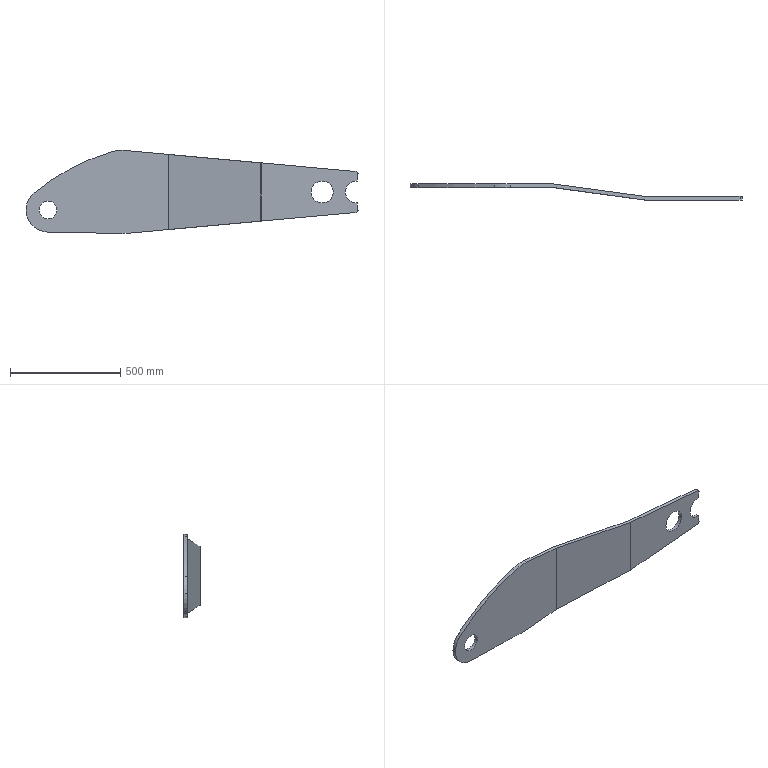Part | SolidWorks | features Extrusion 1, ICE 1 | 1 solid | 28 faces | box 1506 x 73 x 377 mm | volume 6517874 mm3 | cylinder 17 | plane 11 | commonest cylinder face diameters 20 x4 100 x4 52 x2 80 x2 200 x2 377 x2
STEP:
#1=CARTESIAN_POINT('',(-549.379,-8.,118.522));
#2=VERTEX_POINT('',#1);
#3=CARTESIAN_POINT('',(-647.3,-8.,218.5));
#4=VERTEX_POINT('',#3);
#5=CARTESIAN_POINT('',(-547.3,-8.,218.5));
#6=DIRECTION('',(0.,1.,0.));
#7=DIRECTION('',(-1.,0.,0.));
#8=AXIS2_PLACEMENT_3D('',#5,#6,#7);
#9=CIRCLE('',#8,100.);
#10=EDGE_CURVE('',#2,#4,#9,.T.);
#11=ORIENTED_EDGE('',*,*,#10,.T.);
#12=CARTESIAN_POINT('',(-647.3,8.,218.5));
#13=VERTEX_POINT('',#12);
#14=CARTESIAN_POINT('',(-647.3,-65.,218.5));
#15=DIRECTION('',(0.,1.,0.));
#16=VECTOR('',#15,1000.);
#17=LINE('',#14,#16);
#18=EDGE_CURVE('',#4,#13,#17,.T.);
#19=ORIENTED_EDGE('',*,*,#18,.T.);
#20=CARTESIAN_POINT('',(-549.379,8.,118.522));
#21=VERTEX_POINT('',#20);
#22=CARTESIAN_POINT('',(-547.3,8.,218.5));
#23=DIRECTION('',(0.,1.,0.));
#24=DIRECTION('',(-1.,0.,0.));
#25=AXIS2_PLACEMENT_3D('',#22,#23,#24);
#26=CIRCLE('',#25,100.);
#27=EDGE_CURVE('',#21,#13,#26,.T.);
#28=ORIENTED_EDGE('',*,*,#27,.F.);
#29=CARTESIAN_POINT('',(-549.379,-65.,118.522));
#30=DIRECTION('',(0.,1.,0.));
#31=VECTOR('',#30,1000.);
#32=LINE('',#29,#31);
#33=EDGE_CURVE('',#2,#21,#32,.T.);
#34=ORIENTED_EDGE('',*,*,#33,.F.);
#35=EDGE_LOOP('',(#11,#19,#28,#34));
#36=FACE_OUTER_BOUND('',#35,.T.);
#37=CARTESIAN_POINT('',(-547.3,-65.,218.5));
#38=DIRECTION('',(0.,1.,0.));
#39=DIRECTION('',(-1.,0.,0.));
#40=AXIS2_PLACEMENT_3D('',#37,#38,#39);
#41=CYLINDRICAL_SURFACE('',#40,100.);
#42=ADVANCED_FACE('',(#36),#41,.T.);
#43=CARTESIAN_POINT('',(855.554,-65.,349.792));
#44=VERTEX_POINT('',#43);
#45=CARTESIAN_POINT('',(801.,-65.,300.));
#46=VERTEX_POINT('',#45);
#47=CARTESIAN_POINT('',(851.,-65.,300.));
#48=DIRECTION('',(0.,-1.,0.));
#49=DIRECTION('',(-1.,0.,0.));
#50=AXIS2_PLACEMENT_3D('',#47,#48,#49);
#51=CIRCLE('',#50,50.);
#52=EDGE_CURVE('',#44,#46,#51,.T.);
#53=ORIENTED_EDGE('',*,*,#52,.T.);
#54=CARTESIAN_POINT('',(801.,-49.,300.));
#55=VERTEX_POINT('',#54);
#56=CARTESIAN_POINT('',(801.,-65.,300.));
#57=DIRECTION('',(0.,1.,0.));
#58=VECTOR('',#57,1000.);
#59=LINE('',#56,#58);
#60=EDGE_CURVE('',#46,#55,#59,.T.);
#61=ORIENTED_EDGE('',*,*,#60,.T.);
#62=CARTESIAN_POINT('',(855.554,-49.,349.792));
#63=VERTEX_POINT('',#62);
#64=CARTESIAN_POINT('',(851.,-49.,300.));
#65=DIRECTION('',(0.,1.,0.));
#66=DIRECTION('',(0.,0.,-1.));
#67=AXIS2_PLACEMENT_3D('',#64,#65,#66);
#68=CIRCLE('',#67,50.);
#69=EDGE_CURVE('',#55,#63,#68,.T.);
#70=ORIENTED_EDGE('',*,*,#69,.T.);
#71=CARTESIAN_POINT('',(855.554,-65.,349.792));
#72=DIRECTION('',(0.,1.,0.));
#73=VECTOR('',#72,1000.);
#74=LINE('',#71,#73);
#75=EDGE_CURVE('',#44,#63,#74,.T.);
#76=ORIENTED_EDGE('',*,*,#75,.F.);
#77=EDGE_LOOP('',(#53,#61,#70,#76));
#78=FACE_OUTER_BOUND('',#77,.T.);
#79=CARTESIAN_POINT('',(851.,-65.,300.));
#80=DIRECTION('',(0.,1.,0.));
#81=DIRECTION('',(-1.,0.,0.));
#82=AXIS2_PLACEMENT_3D('',#79,#80,#81);
#83=CYLINDRICAL_SURFACE('',#82,50.);
#84=ADVANCED_FACE('',(#78),#83,.F.);
#85=CARTESIAN_POINT('',(746.,-65.,300.));
#86=VERTEX_POINT('',#85);
#87=CARTESIAN_POINT('',(646.,-65.,300.));
#88=VERTEX_POINT('',#87);
#89=CARTESIAN_POINT('',(696.,-65.,300.));
#90=DIRECTION('',(0.,1.,0.));
#91=DIRECTION('',(-1.,0.,0.));
#92=AXIS2_PLACEMENT_3D('',#89,#90,#91);
#93=CIRCLE('',#92,50.);
#94=EDGE_CURVE('',#86,#88,#93,.T.);
#95=ORIENTED_EDGE('',*,*,#94,.F.);
#96=CARTESIAN_POINT('',(746.,-49.,300.));
#97=VERTEX_POINT('',#96);
#98=CARTESIAN_POINT('',(746.,-65.,300.));
#99=DIRECTION('',(0.,1.,0.));
#100=VECTOR('',#99,1000.);
#101=LINE('',#98,#100);
#102=EDGE_CURVE('',#86,#97,#101,.T.);
#103=ORIENTED_EDGE('',*,*,#102,.T.);
#104=CARTESIAN_POINT('',(646.,-49.,300.));
#105=VERTEX_POINT('',#104);
#106=CARTESIAN_POINT('',(696.,-49.,300.));
#107=DIRECTION('',(0.,-1.,0.));
#108=DIRECTION('',(0.,0.,-1.));
#109=AXIS2_PLACEMENT_3D('',#106,#107,#108);
#110=CIRCLE('',#109,50.);
#111=EDGE_CURVE('',#105,#97,#110,.T.);
#112=ORIENTED_EDGE('',*,*,#111,.F.);
#113=CARTESIAN_POINT('',(646.,-65.,300.));
#114=DIRECTION('',(0.,1.,0.));
#115=VECTOR('',#114,1000.);
#116=LINE('',#113,#115);
#117=EDGE_CURVE('',#88,#105,#116,.T.);
#118=ORIENTED_EDGE('',*,*,#117,.F.);
#119=EDGE_LOOP('',(#95,#103,#112,#118));
#120=FACE_OUTER_BOUND('',#119,.T.);
#121=CARTESIAN_POINT('',(696.,-65.,300.));
#122=DIRECTION('',(0.,1.,0.));
#123=DIRECTION('',(-1.,0.,0.));
#124=AXIS2_PLACEMENT_3D('',#121,#122,#123);
#125=CYLINDRICAL_SURFACE('',#124,50.);
#126=ADVANCED_FACE('',(#120),#125,.F.);
#127=CARTESIAN_POINT('',(-507.3,-8.,218.5));
#128=VERTEX_POINT('',#127);
#129=CARTESIAN_POINT('',(-587.3,-8.,218.5));
#130=VERTEX_POINT('',#129);
#131=CARTESIAN_POINT('',(-547.3,-8.,218.5));
#132=DIRECTION('',(0.,1.,0.));
#133=DIRECTION('',(-1.,0.,0.));
#134=AXIS2_PLACEMENT_3D('',#131,#132,#133);
#135=CIRCLE('',#134,40.);
#136=EDGE_CURVE('',#128,#130,#135,.T.);
#137=ORIENTED_EDGE('',*,*,#136,.F.);
#138=CARTESIAN_POINT('',(-507.3,8.,218.5));
#139=VERTEX_POINT('',#138);
#140=CARTESIAN_POINT('',(-507.3,-65.,218.5));
#141=DIRECTION('',(0.,1.,0.));
#142=VECTOR('',#141,1000.);
#143=LINE('',#140,#142);
#144=EDGE_CURVE('',#128,#139,#143,.T.);
#145=ORIENTED_EDGE('',*,*,#144,.T.);
#146=CARTESIAN_POINT('',(-587.3,8.,218.5));
#147=VERTEX_POINT('',#146);
#148=CARTESIAN_POINT('',(-547.3,8.,218.5));
#149=DIRECTION('',(0.,1.,0.));
#150=DIRECTION('',(-1.,0.,0.));
#151=AXIS2_PLACEMENT_3D('',#148,#149,#150);
#152=CIRCLE('',#151,40.);
#153=EDGE_CURVE('',#139,#147,#152,.T.);
#154=ORIENTED_EDGE('',*,*,#153,.T.);
#155=CARTESIAN_POINT('',(-587.3,-65.,218.5));
#156=DIRECTION('',(0.,1.,0.));
#157=VECTOR('',#156,1000.);
#158=LINE('',#155,#157);
#159=EDGE_CURVE('',#130,#147,#158,.T.);
#160=ORIENTED_EDGE('',*,*,#159,.F.);
#161=EDGE_LOOP('',(#137,#145,#154,#160));
#162=FACE_OUTER_BOUND('',#161,.T.);
#163=CARTESIAN_POINT('',(-547.3,-65.,218.5));
#164=DIRECTION('',(0.,1.,0.));
#165=DIRECTION('',(-1.,0.,0.));
#166=AXIS2_PLACEMENT_3D('',#163,#164,#165);
#167=CYLINDRICAL_SURFACE('',#166,40.);
#168=ADVANCED_FACE('',(#162),#167,.F.);
#169=CARTESIAN_POINT('',(-1.216,-8.,470.323));
#170=VERTEX_POINT('',#169);
#171=CARTESIAN_POINT('',(0.129,-8.091,470.2));
#172=VERTEX_POINT('',#171);
#173=CARTESIAN_POINT('',(-1.216,-8.,470.323));
#174=CARTESIAN_POINT('',(-0.7662,-8.,470.282));
#175=CARTESIAN_POINT('',(-0.3171,-8.03,470.241));
#176=CARTESIAN_POINT('',(0.129,-8.091,470.2));
#177=(BOUNDED_CURVE()B_SPLINE_CURVE(3,(#173,#174,#175,#176),.UNSPECIFIED.,.F.,.T.)B_SPLINE_CURVE_WITH_KNOTS((4,4),(4.712,4.847),.UNSPECIFIED.)CURVE()GEOMETRIC_REPRESENTATION_ITEM()RATIONAL_B_SPLINE_CURVE((1.,0.9985,0.9985,1.))REPRESENTATION_ITEM(''));
#178=EDGE_CURVE('',#170,#172,#177,.T.);
#179=ORIENTED_EDGE('',*,*,#178,.F.);
#180=CARTESIAN_POINT('',(-1.216,-8.,129.677));
#181=VERTEX_POINT('',#180);
#182=CARTESIAN_POINT('',(-1.216,-8.,600.));
#183=DIRECTION('',(0.,0.,-1.));
#184=VECTOR('',#183,1000.);
#185=LINE('',#182,#184);
#186=EDGE_CURVE('',#170,#181,#185,.T.);
#187=ORIENTED_EDGE('',*,*,#186,.T.);
#188=CARTESIAN_POINT('',(0.129,-8.091,129.8));
#189=VERTEX_POINT('',#188);
#190=CARTESIAN_POINT('',(0.129,-8.091,129.8));
#191=CARTESIAN_POINT('',(-0.3171,-8.03,129.759));
#192=CARTESIAN_POINT('',(-0.7662,-8.,129.718));
#193=CARTESIAN_POINT('',(-1.216,-8.,129.677));
#194=(BOUNDED_CURVE()B_SPLINE_CURVE(3,(#190,#191,#192,#193),.UNSPECIFIED.,.F.,.T.)B_SPLINE_CURVE_WITH_KNOTS((4,4),(4.577,4.712),.UNSPECIFIED.)CURVE()GEOMETRIC_REPRESENTATION_ITEM()RATIONAL_B_SPLINE_CURVE((1.,0.9985,0.9985,1.))REPRESENTATION_ITEM(''));
#195=EDGE_CURVE('',#189,#181,#194,.T.);
#196=ORIENTED_EDGE('',*,*,#195,.F.);
#197=CARTESIAN_POINT('',(0.129,-8.091,600.));
#198=DIRECTION('',(0.,0.,-1.));
#199=VECTOR('',#198,1000.);
#200=LINE('',#197,#199);
#201=EDGE_CURVE('',#172,#189,#200,.T.);
#202=ORIENTED_EDGE('',*,*,#201,.F.);
#203=EDGE_LOOP('',(#179,#187,#196,#202));
#204=FACE_OUTER_BOUND('',#203,.T.);
#205=CARTESIAN_POINT('',(-1.216,-18.,600.));
#206=DIRECTION('',(0.,0.,-1.));
#207=DIRECTION('',(-1.,0.,0.));
#208=AXIS2_PLACEMENT_3D('',#205,#206,#207);
#209=CYLINDRICAL_SURFACE('',#208,10.);
#210=ADVANCED_FACE('',(#204),#209,.F.);
#211=CARTESIAN_POINT('',(417.518,-64.764,432.272));
#212=VERTEX_POINT('',#211);
#213=CARTESIAN_POINT('',(-11.359,-6.531,471.244));
#214=DIRECTION('',(0.9869,-0.134,-0.08968));
#215=VECTOR('',#214,1000.);
#216=LINE('',#213,#215);
#217=EDGE_CURVE('',#172,#212,#216,.T.);
#218=ORIENTED_EDGE('',*,*,#217,.F.);
#219=ORIENTED_EDGE('',*,*,#201,.T.);
#220=CARTESIAN_POINT('',(417.518,-64.764,167.728));
#221=VERTEX_POINT('',#220);
#222=CARTESIAN_POINT('',(41.746,-13.742,133.581));
#223=DIRECTION('',(-0.9869,0.134,-0.08968));
#224=VECTOR('',#223,1000.);
#225=LINE('',#222,#224);
#226=EDGE_CURVE('',#221,#189,#225,.T.);
#227=ORIENTED_EDGE('',*,*,#226,.F.);
#228=CARTESIAN_POINT('',(417.518,-64.764,600.));
#229=DIRECTION('',(0.,0.,-1.));
#230=VECTOR('',#229,1000.);
#231=LINE('',#228,#230);
#232=EDGE_CURVE('',#212,#221,#231,.T.);
#233=ORIENTED_EDGE('',*,*,#232,.F.);
#234=EDGE_LOOP('',(#218,#219,#227,#233));
#235=FACE_OUTER_BOUND('',#234,.T.);
#236=CARTESIAN_POINT('',(0.129,-8.091,600.));
#237=DIRECTION('',(0.1345,0.9909,0.));
#238=DIRECTION('',(-0.9909,0.1345,0.));
#239=AXIS2_PLACEMENT_3D('',#236,#237,#238);
#240=PLANE('',#239);
#241=ADVANCED_FACE('',(#235),#240,.F.);
#242=CARTESIAN_POINT('',(421.016,-65.,431.954));
#243=VERTEX_POINT('',#242);
#244=CARTESIAN_POINT('',(417.518,-64.764,432.272));
#245=CARTESIAN_POINT('',(418.678,-64.921,432.166));
#246=CARTESIAN_POINT('',(419.846,-65.,432.06));
#247=CARTESIAN_POINT('',(421.016,-65.,431.954));
#248=(BOUNDED_CURVE()B_SPLINE_CURVE(3,(#244,#245,#246,#247),.UNSPECIFIED.,.F.,.T.)B_SPLINE_CURVE_WITH_KNOTS((4,4),(4.577,4.712),.UNSPECIFIED.)CURVE()GEOMETRIC_REPRESENTATION_ITEM()RATIONAL_B_SPLINE_CURVE((1.,0.9985,0.9985,1.))REPRESENTATION_ITEM(''));
#249=EDGE_CURVE('',#212,#243,#248,.T.);
#250=ORIENTED_EDGE('',*,*,#249,.F.);
#251=ORIENTED_EDGE('',*,*,#232,.T.);
#252=CARTESIAN_POINT('',(421.016,-65.,168.046));
#253=VERTEX_POINT('',#252);
#254=CARTESIAN_POINT('',(421.016,-65.,168.046));
#255=CARTESIAN_POINT('',(419.846,-65.,167.94));
#256=CARTESIAN_POINT('',(418.678,-64.921,167.834));
#257=CARTESIAN_POINT('',(417.518,-64.764,167.728));
#258=(BOUNDED_CURVE()B_SPLINE_CURVE(3,(#254,#255,#256,#257),.UNSPECIFIED.,.F.,.T.)B_SPLINE_CURVE_WITH_KNOTS((4,4),(4.712,4.847),.UNSPECIFIED.)CURVE()GEOMETRIC_REPRESENTATION_ITEM()RATIONAL_B_SPLINE_CURVE((1.,0.9985,0.9985,1.))REPRESENTATION_ITEM(''));
#259=EDGE_CURVE('',#253,#221,#258,.T.);
#260=ORIENTED_EDGE('',*,*,#259,.F.);
#261=CARTESIAN_POINT('',(421.016,-65.,600.));
#262=DIRECTION('',(0.,0.,-1.));
#263=VECTOR('',#262,1000.);
#264=LINE('',#261,#263);
#265=EDGE_CURVE('',#243,#253,#264,.T.);
#266=ORIENTED_EDGE('',*,*,#265,.F.);
#267=EDGE_LOOP('',(#250,#251,#260,#266));
#268=FACE_OUTER_BOUND('',#267,.T.);
#269=CARTESIAN_POINT('',(421.016,-39.,600.));
#270=DIRECTION('',(0.,0.,-1.));
#271=DIRECTION('',(-1.,0.,0.));
#272=AXIS2_PLACEMENT_3D('',#269,#270,#271);
#273=CYLINDRICAL_SURFACE('',#272,26.);
#274=ADVANCED_FACE('',(#268),#273,.T.);
#275=CARTESIAN_POINT('',(696.,-65.,300.));
#276=DIRECTION('',(0.,1.,0.));
#277=DIRECTION('',(-1.,0.,0.));
#278=AXIS2_PLACEMENT_3D('',#275,#276,#277);
#279=CIRCLE('',#278,50.);
#280=EDGE_CURVE('',#88,#86,#279,.T.);
#281=ORIENTED_EDGE('',*,*,#280,.T.);
#282=ORIENTED_EDGE('',*,*,#94,.T.);
#283=EDGE_LOOP('',(#281,#282));
#284=FACE_BOUND('',#283,.T.);
#285=CARTESIAN_POINT('',(849.441,-65.,393.023));
#286=VERTEX_POINT('',#285);
#287=CARTESIAN_POINT('',(849.441,-65.,393.023));
#288=DIRECTION('',(0.9959,0.,-0.0905));
#289=VECTOR('',#288,1000.);
#290=LINE('',#287,#289);
#291=EDGE_CURVE('',#243,#286,#290,.T.);
#292=ORIENTED_EDGE('',*,*,#291,.F.);
#293=ORIENTED_EDGE('',*,*,#265,.T.);
#294=CARTESIAN_POINT('',(849.441,-65.,206.977));
#295=VERTEX_POINT('',#294);
#296=CARTESIAN_POINT('',(849.441,-65.,206.977));
#297=DIRECTION('',(-0.9959,0.,-0.0905));
#298=VECTOR('',#297,1000.);
#299=LINE('',#296,#298);
#300=EDGE_CURVE('',#295,#253,#299,.T.);
#301=ORIENTED_EDGE('',*,*,#300,.F.);
#302=CARTESIAN_POINT('',(858.495,-65.,217.841));
#303=VERTEX_POINT('',#302);
#304=CARTESIAN_POINT('',(848.536,-65.,216.936));
#305=DIRECTION('',(0.,1.,0.));
#306=DIRECTION('',(1.,0.,0.));
#307=AXIS2_PLACEMENT_3D('',#304,#305,#306);
#308=CIRCLE('',#307,10.);
#309=EDGE_CURVE('',#303,#295,#308,.T.);
#310=ORIENTED_EDGE('',*,*,#309,.F.);
#311=CARTESIAN_POINT('',(855.554,-65.,250.208));
#312=VERTEX_POINT('',#311);
#313=CARTESIAN_POINT('',(858.495,-65.,217.841));
#314=DIRECTION('',(0.0905,0.,-0.9959));
#315=VECTOR('',#314,1000.);
#316=LINE('',#313,#315);
#317=EDGE_CURVE('',#312,#303,#316,.T.);
#318=ORIENTED_EDGE('',*,*,#317,.F.);
#319=CARTESIAN_POINT('',(851.,-65.,300.));
#320=DIRECTION('',(0.,-1.,0.));
#321=DIRECTION('',(-1.,0.,0.));
#322=AXIS2_PLACEMENT_3D('',#319,#320,#321);
#323=CIRCLE('',#322,50.);
#324=EDGE_CURVE('',#46,#312,#323,.T.);
#325=ORIENTED_EDGE('',*,*,#324,.F.);
#326=ORIENTED_EDGE('',*,*,#52,.F.);
#327=CARTESIAN_POINT('',(858.495,-65.,382.159));
#328=VERTEX_POINT('',#327);
#329=CARTESIAN_POINT('',(858.495,-65.,382.159));
#330=DIRECTION('',(-0.0905,0.,-0.9959));
#331=VECTOR('',#330,1000.);
#332=LINE('',#329,#331);
#333=EDGE_CURVE('',#328,#44,#332,.T.);
#334=ORIENTED_EDGE('',*,*,#333,.F.);
#335=CARTESIAN_POINT('',(848.536,-65.,383.064));
#336=DIRECTION('',(0.,1.,0.));
#337=DIRECTION('',(-1.,0.,0.));
#338=AXIS2_PLACEMENT_3D('',#335,#336,#337);
#339=CIRCLE('',#338,10.);
#340=EDGE_CURVE('',#286,#328,#339,.T.);
#341=ORIENTED_EDGE('',*,*,#340,.F.);
#342=EDGE_LOOP('',(#292,#293,#301,#310,#318,#325,#326,#334,#341));
#343=FACE_OUTER_BOUND('',#342,.T.);
#344=CARTESIAN_POINT('',(421.016,-65.,600.));
#345=DIRECTION('',(0.,1.,0.));
#346=DIRECTION('',(-1.,0.,0.));
#347=AXIS2_PLACEMENT_3D('',#344,#345,#346);
#348=PLANE('',#347);
#349=ADVANCED_FACE('',(#284,#343),#348,.F.);
#350=ORIENTED_EDGE('',*,*,#111,.T.);
#351=CARTESIAN_POINT('',(696.,-49.,300.));
#352=DIRECTION('',(0.,-1.,0.));
#353=DIRECTION('',(0.,0.,-1.));
#354=AXIS2_PLACEMENT_3D('',#351,#352,#353);
#355=CIRCLE('',#354,50.);
#356=EDGE_CURVE('',#97,#105,#355,.T.);
#357=ORIENTED_EDGE('',*,*,#356,.T.);
#358=EDGE_LOOP('',(#350,#357));
#359=FACE_BOUND('',#358,.T.);
#360=CARTESIAN_POINT('',(849.441,-49.,393.023));
#361=VERTEX_POINT('',#360);
#362=CARTESIAN_POINT('',(421.016,-49.,431.954));
#363=VERTEX_POINT('',#362);
#364=CARTESIAN_POINT('',(405.871,-49.,433.33));
#365=DIRECTION('',(-0.9959,0.,0.0905));
#366=VECTOR('',#365,1000.);
#367=LINE('',#364,#366);
#368=EDGE_CURVE('',#361,#363,#367,.T.);
#369=ORIENTED_EDGE('',*,*,#368,.F.);
#370=CARTESIAN_POINT('',(858.495,-49.,382.159));
#371=VERTEX_POINT('',#370);
#372=CARTESIAN_POINT('',(848.536,-49.,383.064));
#373=DIRECTION('',(0.,-1.,0.));
#374=DIRECTION('',(0.,0.,-1.));
#375=AXIS2_PLACEMENT_3D('',#372,#373,#374);
#376=CIRCLE('',#375,10.);
#377=EDGE_CURVE('',#371,#361,#376,.T.);
#378=ORIENTED_EDGE('',*,*,#377,.F.);
#379=CARTESIAN_POINT('',(874.545,-49.,558.788));
#380=DIRECTION('',(0.0905,0.,0.9959));
#381=VECTOR('',#380,1000.);
#382=LINE('',#379,#381);
#383=EDGE_CURVE('',#63,#371,#382,.T.);
#384=ORIENTED_EDGE('',*,*,#383,.F.);
#385=ORIENTED_EDGE('',*,*,#69,.F.);
#386=CARTESIAN_POINT('',(855.554,-49.,250.208));
#387=VERTEX_POINT('',#386);
#388=CARTESIAN_POINT('',(851.,-49.,300.));
#389=DIRECTION('',(0.,1.,0.));
#390=DIRECTION('',(0.,0.,-1.));
#391=AXIS2_PLACEMENT_3D('',#388,#389,#390);
#392=CIRCLE('',#391,50.);
#393=EDGE_CURVE('',#387,#55,#392,.T.);
#394=ORIENTED_EDGE('',*,*,#393,.F.);
#395=CARTESIAN_POINT('',(858.495,-49.,217.841));
#396=VERTEX_POINT('',#395);
#397=CARTESIAN_POINT('',(820.47,-49.,636.299));
#398=DIRECTION('',(-0.0905,0.,0.9959));
#399=VECTOR('',#398,1000.);
#400=LINE('',#397,#399);
#401=EDGE_CURVE('',#396,#387,#400,.T.);
#402=ORIENTED_EDGE('',*,*,#401,.F.);
#403=CARTESIAN_POINT('',(849.441,-49.,206.977));
#404=VERTEX_POINT('',#403);
#405=CARTESIAN_POINT('',(848.536,-49.,216.936));
#406=DIRECTION('',(0.,-1.,0.));
#407=DIRECTION('',(0.,0.,-1.));
#408=AXIS2_PLACEMENT_3D('',#405,#406,#407);
#409=CIRCLE('',#408,10.);
#410=EDGE_CURVE('',#404,#396,#409,.T.);
#411=ORIENTED_EDGE('',*,*,#410,.F.);
#412=CARTESIAN_POINT('',(421.016,-49.,168.046));
#413=VERTEX_POINT('',#412);
#414=CARTESIAN_POINT('',(459.947,-49.,171.584));
#415=DIRECTION('',(0.9959,0.,0.0905));
#416=VECTOR('',#415,1000.);
#417=LINE('',#414,#416);
#418=EDGE_CURVE('',#413,#404,#417,.T.);
#419=ORIENTED_EDGE('',*,*,#418,.F.);
#420=CARTESIAN_POINT('',(421.016,-49.,600.));
#421=DIRECTION('',(0.,0.,-1.));
#422=VECTOR('',#421,1000.);
#423=LINE('',#420,#422);
#424=EDGE_CURVE('',#363,#413,#423,.T.);
#425=ORIENTED_EDGE('',*,*,#424,.F.);
#426=EDGE_LOOP('',(#369,#378,#384,#385,#394,#402,#411,#419,#425));
#427=FACE_OUTER_BOUND('',#426,.T.);
#428=CARTESIAN_POINT('',(421.016,-49.,600.));
#429=DIRECTION('',(0.,-1.,0.));
#430=DIRECTION('',(0.,0.,-1.));
#431=AXIS2_PLACEMENT_3D('',#428,#429,#430);
#432=PLANE('',#431);
#433=ADVANCED_FACE('',(#359,#427),#432,.F.);
#434=CARTESIAN_POINT('',(419.671,-48.909,432.076));
#435=VERTEX_POINT('',#434);
#436=CARTESIAN_POINT('',(421.016,-49.,431.954));
#437=CARTESIAN_POINT('',(420.566,-49.,431.995));
#438=CARTESIAN_POINT('',(420.117,-48.97,432.036));
#439=CARTESIAN_POINT('',(419.671,-48.909,432.076));
#440=(BOUNDED_CURVE()B_SPLINE_CURVE(3,(#436,#437,#438,#439),.UNSPECIFIED.,.F.,.T.)B_SPLINE_CURVE_WITH_KNOTS((4,4),(1.571,1.706),.UNSPECIFIED.)CURVE()GEOMETRIC_REPRESENTATION_ITEM()RATIONAL_B_SPLINE_CURVE((1.,0.9985,0.9985,1.))REPRESENTATION_ITEM(''));
#441=EDGE_CURVE('',#363,#435,#440,.T.);
#442=ORIENTED_EDGE('',*,*,#441,.F.);
#443=ORIENTED_EDGE('',*,*,#424,.T.);
#444=CARTESIAN_POINT('',(419.671,-48.909,167.924));
#445=VERTEX_POINT('',#444);
#446=CARTESIAN_POINT('',(419.671,-48.909,167.924));
#447=CARTESIAN_POINT('',(420.117,-48.97,167.964));
#448=CARTESIAN_POINT('',(420.566,-49.,168.005));
#449=CARTESIAN_POINT('',(421.016,-49.,168.046));
#450=(BOUNDED_CURVE()B_SPLINE_CURVE(3,(#446,#447,#448,#449),.UNSPECIFIED.,.F.,.T.)B_SPLINE_CURVE_WITH_KNOTS((4,4),(1.436,1.571),.UNSPECIFIED.)CURVE()GEOMETRIC_REPRESENTATION_ITEM()RATIONAL_B_SPLINE_CURVE((1.,0.9985,0.9985,1.))REPRESENTATION_ITEM(''));
#451=EDGE_CURVE('',#445,#413,#450,.T.);
#452=ORIENTED_EDGE('',*,*,#451,.F.);
#453=CARTESIAN_POINT('',(419.671,-48.909,600.));
#454=DIRECTION('',(0.,0.,-1.));
#455=VECTOR('',#454,1000.);
#456=LINE('',#453,#455);
#457=EDGE_CURVE('',#435,#445,#456,.T.);
#458=ORIENTED_EDGE('',*,*,#457,.F.);
#459=EDGE_LOOP('',(#442,#443,#452,#458));
#460=FACE_OUTER_BOUND('',#459,.T.);
#461=CARTESIAN_POINT('',(421.016,-39.,600.));
#462=DIRECTION('',(0.,0.,-1.));
#463=DIRECTION('',(-1.,0.,0.));
#464=AXIS2_PLACEMENT_3D('',#461,#462,#463);
#465=CYLINDRICAL_SURFACE('',#464,10.);
#466=ADVANCED_FACE('',(#460),#465,.F.);
#467=CARTESIAN_POINT('',(2.282,7.764,470.005));
#468=VERTEX_POINT('',#467);
#469=CARTESIAN_POINT('',(-9.224,9.326,471.05));
#470=DIRECTION('',(-0.9869,0.134,0.08968));
#471=VECTOR('',#470,1000.);
#472=LINE('',#469,#471);
#473=EDGE_CURVE('',#435,#468,#472,.T.);
#474=ORIENTED_EDGE('',*,*,#473,.F.);
#475=ORIENTED_EDGE('',*,*,#457,.T.);
#476=CARTESIAN_POINT('',(2.282,7.764,129.995));
#477=VERTEX_POINT('',#476);
#478=CARTESIAN_POINT('',(43.881,2.115,133.775));
#479=DIRECTION('',(0.9869,-0.134,0.08968));
#480=VECTOR('',#479,1000.);
#481=LINE('',#478,#480);
#482=EDGE_CURVE('',#477,#445,#481,.T.);
#483=ORIENTED_EDGE('',*,*,#482,.F.);
#484=CARTESIAN_POINT('',(2.282,7.764,600.));
#485=DIRECTION('',(0.,0.,-1.));
#486=VECTOR('',#485,1000.);
#487=LINE('',#484,#486);
#488=EDGE_CURVE('',#468,#477,#487,.T.);
#489=ORIENTED_EDGE('',*,*,#488,.F.);
#490=EDGE_LOOP('',(#474,#475,#483,#489));
#491=FACE_OUTER_BOUND('',#490,.T.);
#492=CARTESIAN_POINT('',(2.282,7.764,600.));
#493=DIRECTION('',(-0.1345,-0.9909,0.));
#494=DIRECTION('',(0.9909,-0.1345,0.));
#495=AXIS2_PLACEMENT_3D('',#492,#493,#494);
#496=PLANE('',#495);
#497=ADVANCED_FACE('',(#491),#496,.F.);
#498=CARTESIAN_POINT('',(-1.216,8.,470.323));
#499=VERTEX_POINT('',#498);
#500=CARTESIAN_POINT('',(2.282,7.764,470.005));
#501=CARTESIAN_POINT('',(1.122,7.921,470.11));
#502=CARTESIAN_POINT('',(-0.04594,8.,470.216));
#503=CARTESIAN_POINT('',(-1.216,8.,470.323));
#504=(BOUNDED_CURVE()B_SPLINE_CURVE(3,(#500,#501,#502,#503),.UNSPECIFIED.,.F.,.T.)B_SPLINE_CURVE_WITH_KNOTS((4,4),(1.436,1.571),.UNSPECIFIED.)CURVE()GEOMETRIC_REPRESENTATION_ITEM()RATIONAL_B_SPLINE_CURVE((1.,0.9985,0.9985,1.))REPRESENTATION_ITEM(''));
#505=EDGE_CURVE('',#468,#499,#504,.T.);
#506=ORIENTED_EDGE('',*,*,#505,.F.);
#507=ORIENTED_EDGE('',*,*,#488,.T.);
#508=CARTESIAN_POINT('',(-1.216,8.,129.677));
#509=VERTEX_POINT('',#508);
#510=CARTESIAN_POINT('',(-1.216,8.,129.677));
#511=CARTESIAN_POINT('',(-0.04594,8.,129.784));
#512=CARTESIAN_POINT('',(1.122,7.921,129.89));
#513=CARTESIAN_POINT('',(2.282,7.764,129.995));
#514=(BOUNDED_CURVE()B_SPLINE_CURVE(3,(#510,#511,#512,#513),.UNSPECIFIED.,.F.,.T.)B_SPLINE_CURVE_WITH_KNOTS((4,4),(1.571,1.706),.UNSPECIFIED.)CURVE()GEOMETRIC_REPRESENTATION_ITEM()RATIONAL_B_SPLINE_CURVE((1.,0.9985,0.9985,1.))REPRESENTATION_ITEM(''));
#515=EDGE_CURVE('',#509,#477,#514,.T.);
#516=ORIENTED_EDGE('',*,*,#515,.F.);
#517=CARTESIAN_POINT('',(-1.216,8.,600.));
#518=DIRECTION('',(0.,0.,-1.));
#519=VECTOR('',#518,1000.);
#520=LINE('',#517,#519);
#521=EDGE_CURVE('',#499,#509,#520,.T.);
#522=ORIENTED_EDGE('',*,*,#521,.F.);
#523=EDGE_LOOP('',(#506,#507,#516,#522));
#524=FACE_OUTER_BOUND('',#523,.T.);
#525=CARTESIAN_POINT('',(-1.216,-18.,600.));
#526=DIRECTION('',(0.,0.,-1.));
#527=DIRECTION('',(-1.,0.,0.));
#528=AXIS2_PLACEMENT_3D('',#525,#526,#527);
#529=CYLINDRICAL_SURFACE('',#528,26.);
#530=ADVANCED_FACE('',(#524),#529,.T.);
#531=CARTESIAN_POINT('',(-547.3,8.,218.5));
#532=DIRECTION('',(0.,1.,0.));
#533=DIRECTION('',(-1.,0.,0.));
#534=AXIS2_PLACEMENT_3D('',#531,#532,#533);
#535=CIRCLE('',#534,40.);
#536=EDGE_CURVE('',#147,#139,#535,.T.);
#537=ORIENTED_EDGE('',*,*,#536,.F.);
#538=ORIENTED_EDGE('',*,*,#153,.F.);
#539=EDGE_LOOP('',(#537,#538));
#540=FACE_BOUND('',#539,.T.);
#541=CARTESIAN_POINT('',(-192.741,8.,487.727));
#542=VERTEX_POINT('',#541);
#543=CARTESIAN_POINT('',(849.441,8.,393.023));
#544=DIRECTION('',(0.9959,0.,-0.0905));
#545=VECTOR('',#544,1000.);
#546=LINE('',#543,#545);
#547=EDGE_CURVE('',#542,#499,#546,.T.);
#548=ORIENTED_EDGE('',*,*,#547,.T.);
#549=ORIENTED_EDGE('',*,*,#521,.T.);
#550=CARTESIAN_POINT('',(-192.741,8.,112.273));
#551=VERTEX_POINT('',#550);
#552=CARTESIAN_POINT('',(849.441,8.,206.977));
#553=DIRECTION('',(-0.9959,0.,-0.0905));
#554=VECTOR('',#553,1000.);
#555=LINE('',#552,#554);
#556=EDGE_CURVE('',#509,#551,#555,.T.);
#557=ORIENTED_EDGE('',*,*,#556,.T.);
#558=CARTESIAN_POINT('',(-213.719,8.,111.541));
#559=VERTEX_POINT('',#558);
#560=CARTESIAN_POINT('',(-209.8,8.,300.));
#561=DIRECTION('',(0.,1.,0.));
#562=DIRECTION('',(-1.,0.,0.));
#563=AXIS2_PLACEMENT_3D('',#560,#561,#562);
#564=CIRCLE('',#563,188.5);
#565=EDGE_CURVE('',#551,#559,#564,.T.);
#566=ORIENTED_EDGE('',*,*,#565,.T.);
#567=CARTESIAN_POINT('',(-549.379,8.,118.522));
#568=DIRECTION('',(-0.9998,0.,0.02079));
#569=VECTOR('',#568,1000.);
#570=LINE('',#567,#569);
#571=EDGE_CURVE('',#559,#21,#570,.T.);
#572=ORIENTED_EDGE('',*,*,#571,.T.);
#573=ORIENTED_EDGE('',*,*,#27,.T.);
#574=CARTESIAN_POINT('',(-610.742,8.,295.798));
#575=VERTEX_POINT('',#574);
#576=CARTESIAN_POINT('',(-547.3,8.,218.5));
#577=DIRECTION('',(0.,1.,0.));
#578=DIRECTION('',(-1.,0.,0.));
#579=AXIS2_PLACEMENT_3D('',#576,#577,#578);
#580=CIRCLE('',#579,100.);
#581=EDGE_CURVE('',#13,#575,#580,.T.);
#582=ORIENTED_EDGE('',*,*,#581,.T.);
#583=CARTESIAN_POINT('',(-264.035,8.,480.529));
#584=VERTEX_POINT('',#583);
#585=CARTESIAN_POINT('',(23.682,8.,-477.186));
#586=DIRECTION('',(0.,1.,0.));
#587=DIRECTION('',(-1.,0.,0.));
#588=AXIS2_PLACEMENT_3D('',#585,#586,#587);
#589=CIRCLE('',#588,1000.);
#590=EDGE_CURVE('',#575,#584,#589,.T.);
#591=ORIENTED_EDGE('',*,*,#590,.T.);
#592=CARTESIAN_POINT('',(-209.8,8.,300.));
#593=DIRECTION('',(0.,1.,0.));
#594=DIRECTION('',(-1.,0.,0.));
#595=AXIS2_PLACEMENT_3D('',#592,#593,#594);
#596=CIRCLE('',#595,188.5);
#597=EDGE_CURVE('',#584,#542,#596,.T.);
#598=ORIENTED_EDGE('',*,*,#597,.T.);
#599=EDGE_LOOP('',(#548,#549,#557,#566,#572,#573,#582,#591,#598));
#600=FACE_OUTER_BOUND('',#599,.T.);
#601=CARTESIAN_POINT('',(-1.216,8.,600.));
#602=DIRECTION('',(0.,-1.,0.));
#603=DIRECTION('',(1.,0.,0.));
#604=AXIS2_PLACEMENT_3D('',#601,#602,#603);
#605=PLANE('',#604);
#606=ADVANCED_FACE('',(#540,#600),#605,.F.);
#607=CARTESIAN_POINT('',(-547.3,-8.,218.5));
#608=DIRECTION('',(0.,1.,0.));
#609=DIRECTION('',(-1.,0.,0.));
#610=AXIS2_PLACEMENT_3D('',#607,#608,#609);
#611=CIRCLE('',#610,40.);
#612=EDGE_CURVE('',#130,#128,#611,.T.);
#613=ORIENTED_EDGE('',*,*,#612,.T.);
#614=ORIENTED_EDGE('',*,*,#136,.T.);
#615=EDGE_LOOP('',(#613,#614));
#616=FACE_BOUND('',#615,.T.);
#617=CARTESIAN_POINT('',(-192.741,-8.,487.727));
#618=VERTEX_POINT('',#617);
#619=CARTESIAN_POINT('',(-12.904,-8.,471.385));
#620=DIRECTION('',(0.9959,0.,-0.0905));
#621=VECTOR('',#620,1000.);
#622=LINE('',#619,#621);
#623=EDGE_CURVE('',#618,#170,#622,.T.);
#624=ORIENTED_EDGE('',*,*,#623,.F.);
#625=CARTESIAN_POINT('',(-264.035,-8.,480.529));
#626=VERTEX_POINT('',#625);
#627=CARTESIAN_POINT('',(-209.8,-8.,300.));
#628=DIRECTION('',(0.,1.,0.));
#629=DIRECTION('',(-1.,0.,0.));
#630=AXIS2_PLACEMENT_3D('',#627,#628,#629);
#631=CIRCLE('',#630,188.5);
#632=EDGE_CURVE('',#626,#618,#631,.T.);
#633=ORIENTED_EDGE('',*,*,#632,.F.);
#634=CARTESIAN_POINT('',(-610.742,-8.,295.798));
#635=VERTEX_POINT('',#634);
#636=CARTESIAN_POINT('',(23.682,-8.,-477.186));
#637=DIRECTION('',(0.,1.,0.));
#638=DIRECTION('',(-1.,0.,0.));
#639=AXIS2_PLACEMENT_3D('',#636,#637,#638);
#640=CIRCLE('',#639,1000.);
#641=EDGE_CURVE('',#635,#626,#640,.T.);
#642=ORIENTED_EDGE('',*,*,#641,.F.);
#643=CARTESIAN_POINT('',(-547.3,-8.,218.5));
#644=DIRECTION('',(0.,1.,0.));
#645=DIRECTION('',(-1.,0.,0.));
#646=AXIS2_PLACEMENT_3D('',#643,#644,#645);
#647=CIRCLE('',#646,100.);
#648=EDGE_CURVE('',#4,#635,#647,.T.);
#649=ORIENTED_EDGE('',*,*,#648,.F.);
#650=ORIENTED_EDGE('',*,*,#10,.F.);
#651=CARTESIAN_POINT('',(-213.719,-8.,111.541));
#652=VERTEX_POINT('',#651);
#653=CARTESIAN_POINT('',(-11.463,-8.,107.334));
#654=DIRECTION('',(-0.9998,0.,0.02079));
#655=VECTOR('',#654,1000.);
#656=LINE('',#653,#655);
#657=EDGE_CURVE('',#652,#2,#656,.T.);
#658=ORIENTED_EDGE('',*,*,#657,.F.);
#659=CARTESIAN_POINT('',(-192.741,-8.,112.273));
#660=VERTEX_POINT('',#659);
#661=CARTESIAN_POINT('',(-209.8,-8.,300.));
#662=DIRECTION('',(0.,1.,0.));
#663=DIRECTION('',(-1.,0.,0.));
#664=AXIS2_PLACEMENT_3D('',#661,#662,#663);
#665=CIRCLE('',#664,188.5);
#666=EDGE_CURVE('',#660,#652,#665,.T.);
#667=ORIENTED_EDGE('',*,*,#666,.F.);
#668=CARTESIAN_POINT('',(41.172,-8.,133.529));
#669=DIRECTION('',(-0.9959,0.,-0.0905));
#670=VECTOR('',#669,1000.);
#671=LINE('',#668,#670);
#672=EDGE_CURVE('',#181,#660,#671,.T.);
#673=ORIENTED_EDGE('',*,*,#672,.F.);
#674=ORIENTED_EDGE('',*,*,#186,.F.);
#675=EDGE_LOOP('',(#624,#633,#642,#649,#650,#658,#667,#673,#674));
#676=FACE_OUTER_BOUND('',#675,.T.);
#677=CARTESIAN_POINT('',(-1.216,-8.,600.));
#678=DIRECTION('',(0.,1.,0.));
#679=DIRECTION('',(-1.,0.,0.));
#680=AXIS2_PLACEMENT_3D('',#677,#678,#679);
#681=PLANE('',#680);
#682=ADVANCED_FACE('',(#616,#676),#681,.F.);
#683=ORIENTED_EDGE('',*,*,#144,.F.);
#684=ORIENTED_EDGE('',*,*,#612,.F.);
#685=ORIENTED_EDGE('',*,*,#159,.T.);
#686=ORIENTED_EDGE('',*,*,#536,.T.);
#687=EDGE_LOOP('',(#683,#684,#685,#686));
#688=FACE_OUTER_BOUND('',#687,.T.);
#689=CARTESIAN_POINT('',(-547.3,-65.,218.5));
#690=DIRECTION('',(0.,1.,0.));
#691=DIRECTION('',(-1.,0.,0.));
#692=AXIS2_PLACEMENT_3D('',#689,#690,#691);
#693=CYLINDRICAL_SURFACE('',#692,40.);
#694=ADVANCED_FACE('',(#688),#693,.F.);
#695=ORIENTED_EDGE('',*,*,#102,.F.);
#696=ORIENTED_EDGE('',*,*,#280,.F.);
#697=ORIENTED_EDGE('',*,*,#117,.T.);
#698=ORIENTED_EDGE('',*,*,#356,.F.);
#699=EDGE_LOOP('',(#695,#696,#697,#698));
#700=FACE_OUTER_BOUND('',#699,.T.);
#701=CARTESIAN_POINT('',(696.,-65.,300.));
#702=DIRECTION('',(0.,1.,0.));
#703=DIRECTION('',(-1.,0.,0.));
#704=AXIS2_PLACEMENT_3D('',#701,#702,#703);
#705=CYLINDRICAL_SURFACE('',#704,50.);
#706=ADVANCED_FACE('',(#700),#705,.F.);
#707=ORIENTED_EDGE('',*,*,#60,.F.);
#708=ORIENTED_EDGE('',*,*,#324,.T.);
#709=CARTESIAN_POINT('',(855.554,-65.,250.208));
#710=DIRECTION('',(0.,1.,0.));
#711=VECTOR('',#710,1000.);
#712=LINE('',#709,#711);
#713=EDGE_CURVE('',#312,#387,#712,.T.);
#714=ORIENTED_EDGE('',*,*,#713,.T.);
#715=ORIENTED_EDGE('',*,*,#393,.T.);
#716=EDGE_LOOP('',(#707,#708,#714,#715));
#717=FACE_OUTER_BOUND('',#716,.T.);
#718=CARTESIAN_POINT('',(851.,-65.,300.));
#719=DIRECTION('',(0.,1.,0.));
#720=DIRECTION('',(-1.,0.,0.));
#721=AXIS2_PLACEMENT_3D('',#718,#719,#720);
#722=CYLINDRICAL_SURFACE('',#721,50.);
#723=ADVANCED_FACE('',(#717),#722,.F.);
#724=ORIENTED_EDGE('',*,*,#383,.T.);
#725=CARTESIAN_POINT('',(858.495,-65.,382.159));
#726=DIRECTION('',(0.,1.,0.));
#727=VECTOR('',#726,1000.);
#728=LINE('',#725,#727);
#729=EDGE_CURVE('',#328,#371,#728,.T.);
#730=ORIENTED_EDGE('',*,*,#729,.F.);
#731=ORIENTED_EDGE('',*,*,#333,.T.);
#732=ORIENTED_EDGE('',*,*,#75,.T.);
#733=EDGE_LOOP('',(#724,#730,#731,#732));
#734=FACE_OUTER_BOUND('',#733,.T.);
#735=CARTESIAN_POINT('',(858.495,-65.,382.159));
#736=DIRECTION('',(0.9959,0.,-0.0905));
#737=DIRECTION('',(-0.0905,0.,-0.9959));
#738=AXIS2_PLACEMENT_3D('',#735,#736,#737);
#739=PLANE('',#738);
#740=ADVANCED_FACE('',(#734),#739,.T.);
#741=ORIENTED_EDGE('',*,*,#377,.T.);
#742=CARTESIAN_POINT('',(849.441,-65.,393.023));
#743=DIRECTION('',(0.,1.,0.));
#744=VECTOR('',#743,1000.);
#745=LINE('',#742,#744);
#746=EDGE_CURVE('',#286,#361,#745,.T.);
#747=ORIENTED_EDGE('',*,*,#746,.F.);
#748=ORIENTED_EDGE('',*,*,#340,.T.);
#749=ORIENTED_EDGE('',*,*,#729,.T.);
#750=EDGE_LOOP('',(#741,#747,#748,#749));
#751=FACE_OUTER_BOUND('',#750,.T.);
#752=CARTESIAN_POINT('',(848.536,-65.,383.064));
#753=DIRECTION('',(0.,1.,0.));
#754=DIRECTION('',(-1.,0.,0.));
#755=AXIS2_PLACEMENT_3D('',#752,#753,#754);
#756=CYLINDRICAL_SURFACE('',#755,10.);
#757=ADVANCED_FACE('',(#751),#756,.T.);
#758=ORIENTED_EDGE('',*,*,#410,.T.);
#759=CARTESIAN_POINT('',(858.495,-65.,217.841));
#760=DIRECTION('',(0.,1.,0.));
#761=VECTOR('',#760,1000.);
#762=LINE('',#759,#761);
#763=EDGE_CURVE('',#303,#396,#762,.T.);
#764=ORIENTED_EDGE('',*,*,#763,.F.);
#765=ORIENTED_EDGE('',*,*,#309,.T.);
#766=CARTESIAN_POINT('',(849.441,-65.,206.977));
#767=DIRECTION('',(0.,1.,0.));
#768=VECTOR('',#767,1000.);
#769=LINE('',#766,#768);
#770=EDGE_CURVE('',#295,#404,#769,.T.);
#771=ORIENTED_EDGE('',*,*,#770,.T.);
#772=EDGE_LOOP('',(#758,#764,#765,#771));
#773=FACE_OUTER_BOUND('',#772,.T.);
#774=CARTESIAN_POINT('',(848.536,-65.,216.936));
#775=DIRECTION('',(0.,1.,0.));
#776=DIRECTION('',(-1.,0.,0.));
#777=AXIS2_PLACEMENT_3D('',#774,#775,#776);
#778=CYLINDRICAL_SURFACE('',#777,10.);
#779=ADVANCED_FACE('',(#773),#778,.T.);
#780=ORIENTED_EDGE('',*,*,#401,.T.);
#781=ORIENTED_EDGE('',*,*,#713,.F.);
#782=ORIENTED_EDGE('',*,*,#317,.T.);
#783=ORIENTED_EDGE('',*,*,#763,.T.);
#784=EDGE_LOOP('',(#780,#781,#782,#783));
#785=FACE_OUTER_BOUND('',#784,.T.);
#786=CARTESIAN_POINT('',(858.495,-65.,217.841));
#787=DIRECTION('',(0.9959,0.,0.0905));
#788=DIRECTION('',(0.0905,0.,-0.9959));
#789=AXIS2_PLACEMENT_3D('',#786,#787,#788);
#790=PLANE('',#789);
#791=ADVANCED_FACE('',(#785),#790,.T.);
#792=ORIENTED_EDGE('',*,*,#368,.T.);
#793=ORIENTED_EDGE('',*,*,#441,.T.);
#794=ORIENTED_EDGE('',*,*,#473,.T.);
#795=ORIENTED_EDGE('',*,*,#505,.T.);
#796=ORIENTED_EDGE('',*,*,#547,.F.);
#797=CARTESIAN_POINT('',(-192.741,-65.,487.727));
#798=DIRECTION('',(0.,1.,0.));
#799=VECTOR('',#798,1000.);
#800=LINE('',#797,#799);
#801=EDGE_CURVE('',#618,#542,#800,.T.);
#802=ORIENTED_EDGE('',*,*,#801,.F.);
#803=ORIENTED_EDGE('',*,*,#623,.T.);
#804=ORIENTED_EDGE('',*,*,#178,.T.);
#805=ORIENTED_EDGE('',*,*,#217,.T.);
#806=ORIENTED_EDGE('',*,*,#249,.T.);
#807=ORIENTED_EDGE('',*,*,#291,.T.);
#808=ORIENTED_EDGE('',*,*,#746,.T.);
#809=EDGE_LOOP('',(#792,#793,#794,#795,#796,#802,#803,#804,#805,#806,#807,#808));
#810=FACE_OUTER_BOUND('',#809,.T.);
#811=CARTESIAN_POINT('',(849.441,-65.,393.023));
#812=DIRECTION('',(0.0905,0.,0.9959));
#813=DIRECTION('',(0.9959,0.,-0.0905));
#814=AXIS2_PLACEMENT_3D('',#811,#812,#813);
#815=PLANE('',#814);
#816=ADVANCED_FACE('',(#810),#815,.T.);
#817=ORIENTED_EDGE('',*,*,#632,.T.);
#818=ORIENTED_EDGE('',*,*,#801,.T.);
#819=ORIENTED_EDGE('',*,*,#597,.F.);
#820=CARTESIAN_POINT('',(-264.035,-65.,480.529));
#821=DIRECTION('',(0.,1.,0.));
#822=VECTOR('',#821,1000.);
#823=LINE('',#820,#822);
#824=EDGE_CURVE('',#626,#584,#823,.T.);
#825=ORIENTED_EDGE('',*,*,#824,.F.);
#826=EDGE_LOOP('',(#817,#818,#819,#825));
#827=FACE_OUTER_BOUND('',#826,.T.);
#828=CARTESIAN_POINT('',(-209.8,-65.,300.));
#829=DIRECTION('',(0.,1.,0.));
#830=DIRECTION('',(-1.,0.,0.));
#831=AXIS2_PLACEMENT_3D('',#828,#829,#830);
#832=CYLINDRICAL_SURFACE('',#831,188.5);
#833=ADVANCED_FACE('',(#827),#832,.T.);
#834=ORIENTED_EDGE('',*,*,#641,.T.);
#835=ORIENTED_EDGE('',*,*,#824,.T.);
#836=ORIENTED_EDGE('',*,*,#590,.F.);
#837=CARTESIAN_POINT('',(-610.742,-65.,295.798));
#838=DIRECTION('',(0.,1.,0.));
#839=VECTOR('',#838,1000.);
#840=LINE('',#837,#839);
#841=EDGE_CURVE('',#635,#575,#840,.T.);
#842=ORIENTED_EDGE('',*,*,#841,.F.);
#843=EDGE_LOOP('',(#834,#835,#836,#842));
#844=FACE_OUTER_BOUND('',#843,.T.);
#845=CARTESIAN_POINT('',(23.682,-65.,-477.186));
#846=DIRECTION('',(0.,1.,0.));
#847=DIRECTION('',(-1.,0.,0.));
#848=AXIS2_PLACEMENT_3D('',#845,#846,#847);
#849=CYLINDRICAL_SURFACE('',#848,1000.);
#850=ADVANCED_FACE('',(#844),#849,.T.);
#851=ORIENTED_EDGE('',*,*,#18,.F.);
#852=ORIENTED_EDGE('',*,*,#648,.T.);
#853=ORIENTED_EDGE('',*,*,#841,.T.);
#854=ORIENTED_EDGE('',*,*,#581,.F.);
#855=EDGE_LOOP('',(#851,#852,#853,#854));
#856=FACE_OUTER_BOUND('',#855,.T.);
#857=CARTESIAN_POINT('',(-547.3,-65.,218.5));
#858=DIRECTION('',(0.,1.,0.));
#859=DIRECTION('',(-1.,0.,0.));
#860=AXIS2_PLACEMENT_3D('',#857,#858,#859);
#861=CYLINDRICAL_SURFACE('',#860,100.);
#862=ADVANCED_FACE('',(#856),#861,.T.);
#863=ORIENTED_EDGE('',*,*,#657,.T.);
#864=ORIENTED_EDGE('',*,*,#33,.T.);
#865=ORIENTED_EDGE('',*,*,#571,.F.);
#866=CARTESIAN_POINT('',(-213.719,-65.,111.541));
#867=DIRECTION('',(0.,1.,0.));
#868=VECTOR('',#867,1000.);
#869=LINE('',#866,#868);
#870=EDGE_CURVE('',#652,#559,#869,.T.);
#871=ORIENTED_EDGE('',*,*,#870,.F.);
#872=EDGE_LOOP('',(#863,#864,#865,#871));
#873=FACE_OUTER_BOUND('',#872,.T.);
#874=CARTESIAN_POINT('',(-549.379,-65.,118.522));
#875=DIRECTION('',(-0.02079,0.,-0.9998));
#876=DIRECTION('',(-0.9998,0.,0.02079));
#877=AXIS2_PLACEMENT_3D('',#874,#875,#876);
#878=PLANE('',#877);
#879=ADVANCED_FACE('',(#873),#878,.T.);
#880=ORIENTED_EDGE('',*,*,#666,.T.);
#881=ORIENTED_EDGE('',*,*,#870,.T.);
#882=ORIENTED_EDGE('',*,*,#565,.F.);
#883=CARTESIAN_POINT('',(-192.741,-65.,112.273));
#884=DIRECTION('',(0.,1.,0.));
#885=VECTOR('',#884,1000.);
#886=LINE('',#883,#885);
#887=EDGE_CURVE('',#660,#551,#886,.T.);
#888=ORIENTED_EDGE('',*,*,#887,.F.);
#889=EDGE_LOOP('',(#880,#881,#882,#888));
#890=FACE_OUTER_BOUND('',#889,.T.);
#891=CARTESIAN_POINT('',(-209.8,-65.,300.));
#892=DIRECTION('',(0.,1.,0.));
#893=DIRECTION('',(-1.,0.,0.));
#894=AXIS2_PLACEMENT_3D('',#891,#892,#893);
#895=CYLINDRICAL_SURFACE('',#894,188.5);
#896=ADVANCED_FACE('',(#890),#895,.T.);
#897=ORIENTED_EDGE('',*,*,#418,.T.);
#898=ORIENTED_EDGE('',*,*,#770,.F.);
#899=ORIENTED_EDGE('',*,*,#300,.T.);
#900=ORIENTED_EDGE('',*,*,#259,.T.);
#901=ORIENTED_EDGE('',*,*,#226,.T.);
#902=ORIENTED_EDGE('',*,*,#195,.T.);
#903=ORIENTED_EDGE('',*,*,#672,.T.);
#904=ORIENTED_EDGE('',*,*,#887,.T.);
#905=ORIENTED_EDGE('',*,*,#556,.F.);
#906=ORIENTED_EDGE('',*,*,#515,.T.);
#907=ORIENTED_EDGE('',*,*,#482,.T.);
#908=ORIENTED_EDGE('',*,*,#451,.T.);
#909=EDGE_LOOP('',(#897,#898,#899,#900,#901,#902,#903,#904,#905,#906,#907,#908));
#910=FACE_OUTER_BOUND('',#909,.T.);
#911=CARTESIAN_POINT('',(849.441,-65.,206.977));
#912=DIRECTION('',(0.0905,0.,-0.9959));
#913=DIRECTION('',(-0.9959,0.,-0.0905));
#914=AXIS2_PLACEMENT_3D('',#911,#912,#913);
#915=PLANE('',#914);
#916=ADVANCED_FACE('',(#910),#915,.T.);
#917=CLOSED_SHELL('',(#42,#84,#126,#168,#210,#241,#274,#349,#433,#466,#497,#530,#606,#682,#694,#706,#723,#740,#757,#779,#791,#816,#833,#850,#862,#879,#896,#916));
#918=MANIFOLD_SOLID_BREP('',#917);
#919=CARTESIAN_POINT('',(0.,0.,0.));
#920=DIRECTION('',(0.,0.,1.));
#921=DIRECTION('',(1.,0.,0.));
#922=AXIS2_PLACEMENT_3D('',#919,#920,#921);
#923=(LENGTH_UNIT()NAMED_UNIT(*)SI_UNIT(.MILLI.,.METRE.));
#924=UNCERTAINTY_MEASURE_WITH_UNIT(LENGTH_MEASURE(0.00001),#923,'','');
#925=(NAMED_UNIT(*)PLANE_ANGLE_UNIT()SI_UNIT($,.RADIAN.));
#926=(NAMED_UNIT(*)SI_UNIT($,.STERADIAN.)SOLID_ANGLE_UNIT());
#927=(GEOMETRIC_REPRESENTATION_CONTEXT(3)GLOBAL_UNCERTAINTY_ASSIGNED_CONTEXT((#924))GLOBAL_UNIT_ASSIGNED_CONTEXT((#923,#925,#926))REPRESENTATION_CONTEXT('',''));
#928=ADVANCED_BREP_SHAPE_REPRESENTATION('',(#918,#922),#927);